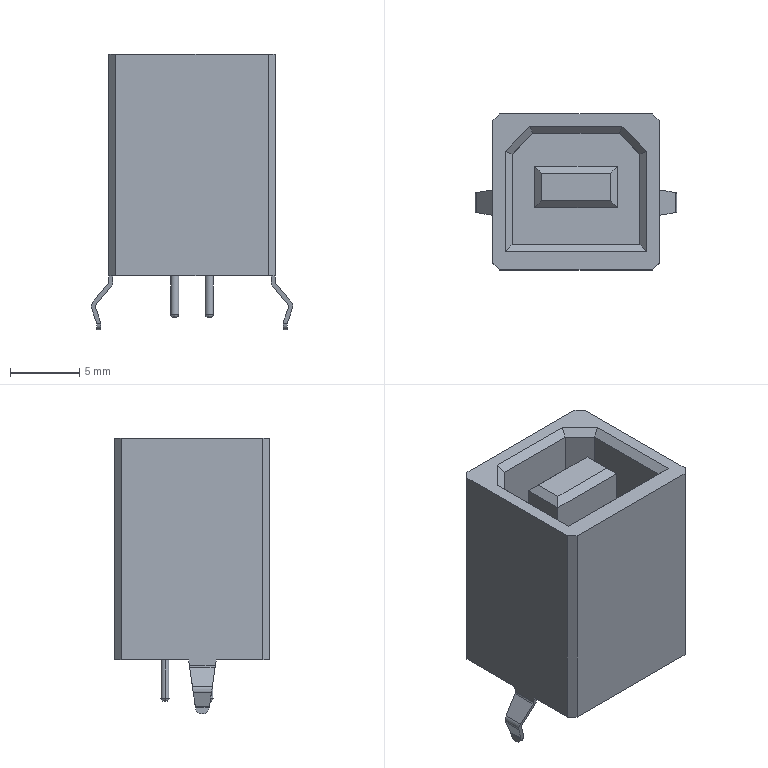Part | SolidWorks | features BaseBody 1 | 1 solid | 86 faces | box 14.571 x 11.26 x 19.95 mm | volume 1672 mm3 | plane 54 | cylinder 24 | spline 8 | commonest cylinder face diameters 1 x10 0.6 x8 0.4 x6